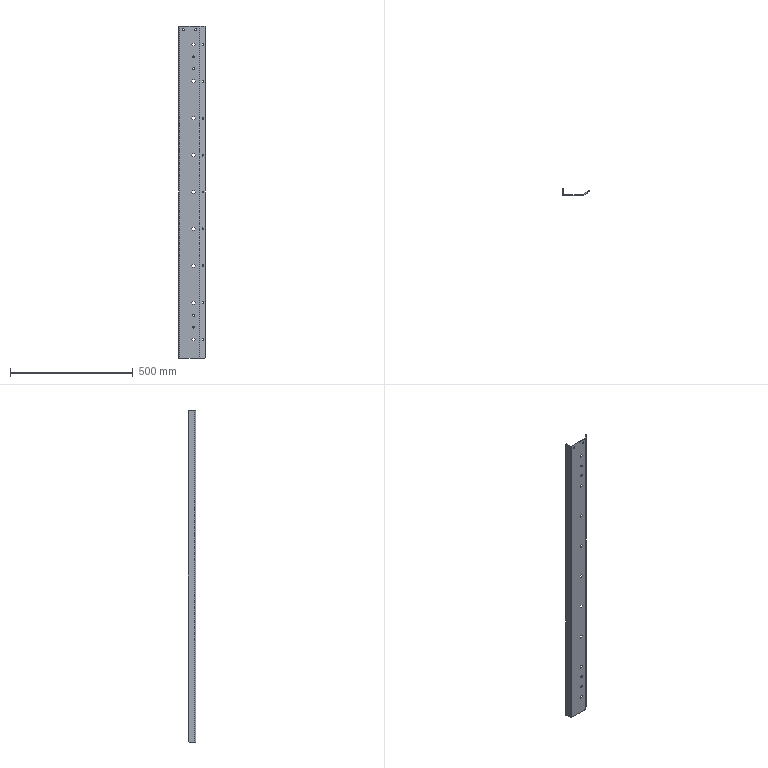Part | STEP file | Side panel wer5 BeforeLift gravity | 1 solid | 95 faces | box 107.981 x 30 x 1350 mm | volume 376755 mm3 | plane 72 | cylinder 23 | commonest cylinder face diameters 8.2 x15 6 x4 4 x2 8 x2